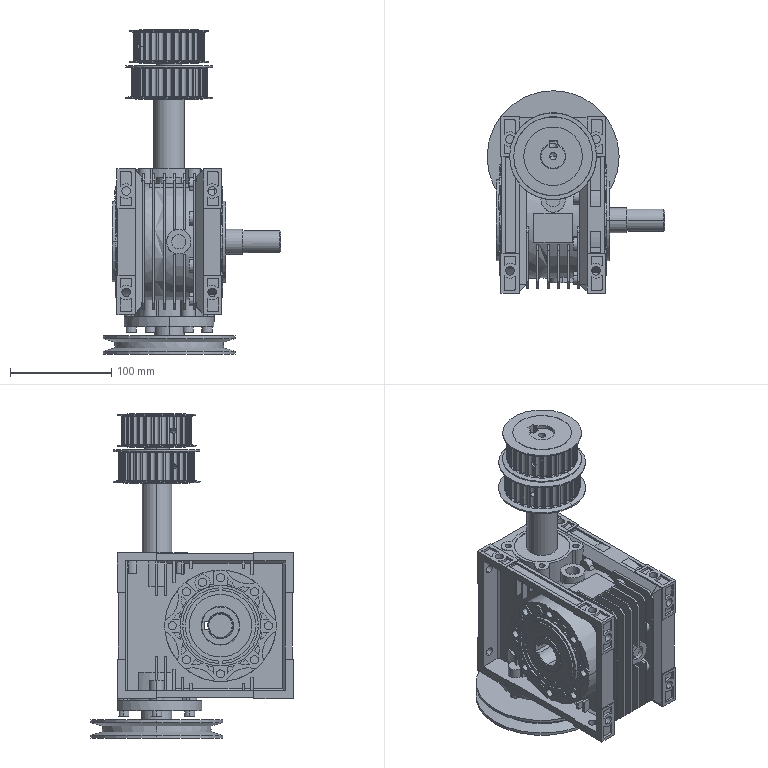Part | SolidWorks | 5 solids | 2352 faces | box 175.75 x 200.25 x 320.306 mm | volume 2291161 mm3 | plane 1250 | cylinder 1029 | cone 45 | spline 28 | commonest cylinder face diameters 1 x148 0.81 x147 8 x63 5.199 x44 5.201 x41 13 x38